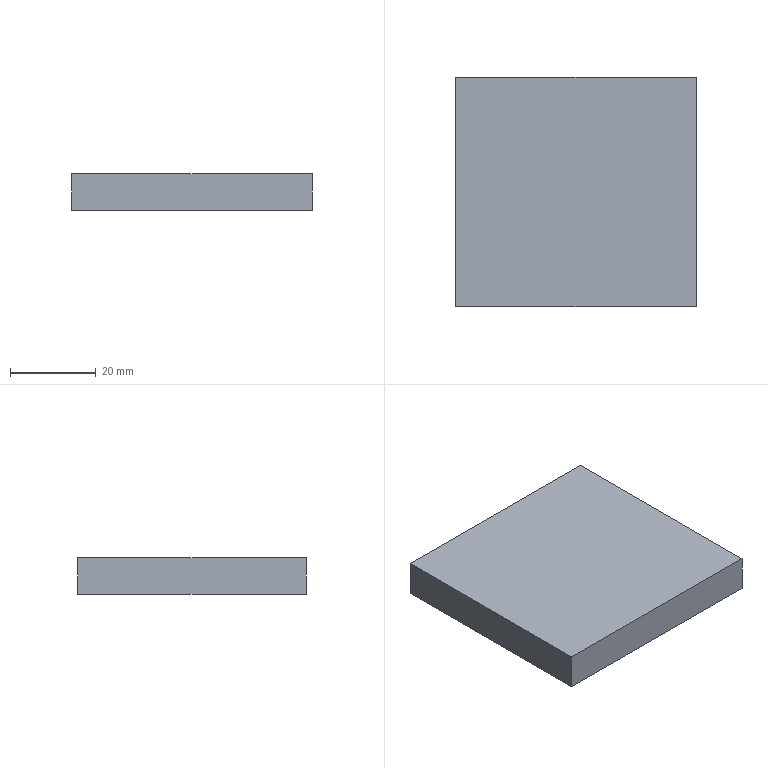NC program | NX | posted with a generic post | part box 56 x 53.3 x 8.5 mm
Lines 1 to 1399 of 2424:
N10 G17 G21 G94 G90
(FLOOR_WALL_COPY , TOOL : D80)
N12 T19 M6
N14 G54
N16 G17 G0 G90 X-73. Y0. S6500 M3
N18 G43 Z30. H19
N20 Z3.
N22 G94 G1 Z0. F1500.
N24 X-68.
N26 X68.
N28 X73.
N30 Z3.
N32 G0 Z30.
N34 M5
(DRILLING_COPY_1 , TOOL : D6A45)
N36 T01 M6
N38 G54
N40 G17 G0 G90 X-16. Y-10. S5000 M3
N42 G43 Z30. H1
N44 G94 G81 G98 Z-1. F350. R3.
N46 X-10.4 Y16.2
N48 X4.1 Y18.5
N50 X16. Y10.
N52 G80
N54 G0 X16. Y10. Z30.
N56 M5
(DRILLING_COPY_1_COPY , TOOL : 2.0ZT)
N58 T16 M6
N60 G54
N62 G17 G0 G90 X4.1 Y18.5 S2000 M3
N64 G43 Z30. H16
N66 G94 G83 G98 Z-3.101 F150. Q2. R3.
N68 X-10.4 Y16.2
N70 G80
N72 G0 X-10.4 Y16.2 Z30.
N74 M5
(DRILLING_COPY_1_COPY_COPY , TOOL : 2.4ZT)
N76 T17 M6
N78 G54
N80 G17 G0 G90 X-16. Y-10. S2000 M3
N82 G43 Z30. H17
N84 G94 G83 G98 Z-5.721 F150. Q2. R3.
N86 X16. Y10.
N88 G80
N90 G0 X16. Y10. Z30.
N92 M5
(ADAPTIVE_MILLING , TOOL : D10)
N94 T15 M6
N96 G54
N98 G17 G0 G90 X-35.709 Y0.039 S9500 M3
N100 G43 Z30. H15
N102 Z-0.5
N104 G94 G1 Z-3.5 F1000.
N106 X-34.928 Y-0.241 F3000.
N108 X-34.14 Y-0.497
N110 G3 X-33.062 Y0.039 R1.017
N112 X-32.301 Y3.102 R8.28
N114 X-32.018 Y12.969 R111.643
N116 G1 X-32.014 Y15.219
N118 X-32.011 Y19.094
N120 X-32.01 Y23.594
N122 X-32.005 Y23.844
N124 X-31.996 Y23.969
N126 X-31.983 Y24.093
N128 G2 X-29.126 Y28.303 R6.082
N130 X-23.363 Y30.215 R13.607
N132 X-14.877 Y30.613 R73.957
N134 G1 X-13.627 Y30.621
N136 X-12.127 Y30.628
N138 X-9.877 Y30.633
N140 X-6.252 Y30.636
N142 X4.748 Y30.638
N144 X24.998
N146 G2 X29.25 Y28.336 R5.606
N148 X31.446 Y22.821 R11.938
N150 X31.954 Y14.47 R57.249
N152 G1 X31.965 Y13.345
N154 X31.973 Y12.095
N156 X31.979 Y10.595
N158 X31.984 Y8.345
N160 X31.987 Y4.47
N162 X31.988 Y-9.155
N164 G2 X31.958 Y-24.154 R786.442
N166 X29.074 Y-28.344 R6.068
N168 X23.298 Y-30.225 R13.818
N170 X14.187 Y-30.618 R81.444
N172 G1 X12.937 Y-30.625
N174 X11.062 Y-30.631
N176 X8.312 Y-30.635
N178 X2.937 Y-30.637
N180 X-25.063 Y-30.638
N182 X-25.188 Y-30.635
N184 G2 X-29.515 Y-27.986 R5.827
N186 X-31.515 Y-22.387 R12.902
N188 X-31.964 Y-13.53 R68.549
N190 X-31.945 Y-2.656 R313.124
N192 G3 X-31.266 Y4.184 R246.26
N194 X-31.025 Y17.68 R253.193
N196 G2 X-30.938 Y21.676 R34.702
N198 X-26.882 Y27.245 R7.984
N200 X-20.34 Y29.196 R16.868
N202 X-10.728 Y29.602 R93.012
N204 G1 X-9.228 Y29.612
N206 X-7.728 Y29.618
N208 X-5.353 Y29.623
N210 X-1.353 Y29.626
N212 X11.272 Y29.627
N214 X21.897
N216 G2 X28.333 Y25.939 R7.618
N218 X30.48 Y19.467 R15.556
N220 X30.949 Y9.86 R80.002
N222 G1 X30.958 Y8.61
N224 X30.966 Y6.985
N226 X30.972 Y4.735
N228 X30.975 Y1.36
N230 X30.977 Y-6.39
N232 Y-20.515
N234 G2 X27.52 Y-26.824 R7.557
N236 X21.095 Y-29.096 R15.023
N238 X11.49 Y-29.597 R73.918
N240 G1 X10.24 Y-29.606
N242 X8.865 Y-29.613
N244 X6.865 Y-29.62
N246 X3.99 Y-29.624
N248 X-1.51 Y-29.626
N250 X-21.885 Y-29.627
N252 G2 X-28.186 Y-26.156 R7.552
N254 X-30.409 Y-19.974 R14.802
N256 X-30.94 Y-10.872 R67.194
N258 X-30.493 Y1.36 R90.695
N260 G3 X-30.042 Y17.349 R205.607
N262 G2 X-28.715 Y22.853 R9.591
N264 X-22.888 Y27.14 R10.859
N266 X-15.391 Y28.397 R28.546
N268 X-1.019 Y28.613 R293.42
N270 G1 X4.106 Y28.615
N272 X19.231 Y28.616
N274 X19.606 Y28.612
N276 X19.731 Y28.609
N278 X19.981 Y28.6
N280 X20.105 Y28.593
N282 G2 X27.438 Y23.856 R8.921
N284 X29.471 Y17.075 R18.202
N286 X29.936 Y7.092 R89.122
N288 G1 X29.946 Y5.842
N290 X29.954 Y4.217
N292 X29.959 Y2.217
N294 X29.964 Y-0.908
N296 X29.966 Y-6.908
N298 Y-17.908
N300 G2 X25.183 Y-26.102 R8.956
N302 X18.028 Y-28.173 R18.615
N304 X8.416 Y-28.587 R94.427
N306 G1 X7.041 Y-28.596
N308 X5.292 Y-28.604
N310 X3.042 Y-28.61
N312 X-0.458 Y-28.614
N314 X-7.833 Y-28.616
N316 X-19.208
N318 G2 X-27.427 Y-23.878 R8.94
N320 X-29.482 Y-16.976 R18.308
N322 X-29.583 Y-0.127 R88.532
N324 G3 X-29.046 Y16.236 R256.072
N326 G2 X-23.515 Y25.097 R9.923
N328 X-16.337 Y27.116 R20.252
N330 X-5.227 Y27.579 R107.451
N332 G1 X-3.727 Y27.588
N334 X-1.852 Y27.595
N336 X0.773 Y27.601
N338 X4.898 Y27.604
N340 X15.898 Y27.605
N342 X17.023
N344 G2 X23.681 Y25.524 R10.12
N346 X27.61 Y19.27 R12.456
N348 X28.753 Y11.497 R33.234
N350 X28.952 Y-3.25 R342.251
N352 X28.926 Y-16.75 R787.554
N354 X23.551 Y-25.057 R9.789
N356 X16.384 Y-27.111 R19.878
N358 X5.275 Y-27.58 R106.924
N360 G1 X3.775 Y-27.589
N362 X1.775 Y-27.596
N364 X-0.975 Y-27.601
N366 X-5.475 Y-27.604
N368 X-16.85 Y-27.605
N370 X-17.225 Y-27.603
N372 G2 X-26.465 Y-22.091 R9.883
N374 X-28.458 Y-15.033 R20.3
N376 X-28.662 Y-1.927 R74.071
N378 G3 X-28.053 Y14.684 R379.618
N380 G2 X-22. Y24.063 R10.638
N382 X-14.44 Y26.108 R21.789
N384 X-3.382 Y26.566 R113.181
N386 X2.387 Y26.68 R28.057
N388 G1 X3.011 Y26.665
N390 X3.636 Y26.654
N392 X4.511 Y26.643
N394 X5.636 Y26.634
N396 X7.136 Y26.627
N398 X9.136 Y26.621
N400 X12.261 Y26.618
N402 X14.011 Y26.616
N404 X14.761 Y26.611
N406 X15.261 Y26.605
N408 X15.511 Y26.6
N410 X15.761 Y26.593
N412 X16.136 Y26.577
N414 G2 X25.417 Y20.594 R10.522
N416 X27.462 Y13.035 R21.667
N418 X27.901 Y3.547 R101.721
N420 X28.033 Y-2.23 R26.861
N422 G1 X28.02 Y-2.73
N424 X28.007 Y-3.354
N426 X28. Y-3.854
N428 X27.989 Y-4.854
N430 X27.981 Y-6.104
N432 X27.974 Y-7.729
N434 X27.97 Y-10.104
N436 X27.967 Y-12.604
N438 X27.962 Y-13.354
N440 X27.954 Y-13.979
N442 X27.948 Y-14.229
N444 X27.935 Y-14.604
N446 X27.929 Y-14.729
N448 G2 X21.883 Y-24.101 R10.563
N450 X14.44 Y-26.105 R21.679
N452 X3.37 Y-26.568 R110.818
N454 X-2.387 Y-26.68 R28.095
N456 G1 X-3.011 Y-26.665
N458 X-3.636 Y-26.654
N460 X-4.511 Y-26.643
N462 X-5.636 Y-26.634
N464 X-7.136 Y-26.627
N466 X-9.136 Y-26.621
N468 X-12.261 Y-26.618
N470 X-14.011 Y-26.616
N472 X-14.761 Y-26.611
N474 X-15.261 Y-26.605
N476 X-15.511 Y-26.6
N478 X-15.886 Y-26.589
N480 X-16.136 Y-26.578
N482 G2 X-25.358 Y-20.705 R10.493
N484 X-27.449 Y-13.159 R21.481
N486 X-27.73 Y-4.617 R60.605
N488 G1 X-27.989 Y-2.991
N490 X-27.995 Y-2.935
N492 G2 X-27.556 Y5.706 R30.137
N494 G3 X-27.106 Y12.94 R98.432
N496 G2 X-24.212 Y20.348 R11.486
N498 X-17.228 Y24.284 R14.404
N500 X-8.567 Y25.4 R40.82
N502 G1 X-8.443 Y25.417
N504 X-5.945 Y26.131
N506 X-5.887 Y26.144
N508 X-3.299 Y26.58
N510 X-2.947 Y26.636
N512 X0.015 Y26.799
N514 X2.947 Y26.636
N516 X3.006 Y26.629
N518 G3 X8.799 Y25.803 R52.382
N520 G2 X15.168 Y25.547 R338.64
N522 X24.383 Y19.168 R11.095
N524 X26.43 Y11.477 R22.827
N526 G3 X26.7 Y8.869 R39.134
N528 G2 X27.904 Y3.531 R28.312
N530 G3 X29.234 Y2.749 R1.003
N532 X29.846 Y3.376 Z-3.455 R1.051
N534 G1 X30.288 Y4.378 Z-3.4
N536 X31.032 Y6.062
N538 G3 X31.086 Y6.713 R1.04
N540 G1 X28.465 Y17.012
N542 G3 X27.102 Y20.468 R15.003
N544 X24.439 Y24.532 R32.276
N546 X21.759 Y26.717 R9.19
N548 X18.514 Y27.978 R14.859
N550 X14.231 Y28.801 R25.607
N552 G1 X9.127 Y29.313
N554 X8.873 Y29.302
N556 X8.627 Y29.234
N558 X6.893 Y28.477
N560 X6.279 Y28.214 Z-3.433
N562 X5.674 Y27.93 Z-3.467
N564 G3 X5.274 Y27.417 Z-3.5 R1.041
N566 X5.945 Y26.131 R1.004
N568 X10.228 Y25.051 R31.02
N570 G2 X15.184 Y24.411 R63.089
N572 X23.404 Y17.715 R11.779
N574 X25.26 Y11.25 R23.658
N576 G3 X26.072 Y10.138 R3.622
N578 G1 X26.147 Y10.022
N580 X26.732 Y8.802
N582 G3 X28.202 Y8.411 R1.004
N584 X28.638 Y9.19 Z-3.454 R1.048
N586 G1 X28.79 Y10.256 Z-3.4
N588 X28.938 Y11.271
N590 X29.07 Y12.289
N592 X29.044 Y12.497
N594 X28.982 Y12.699
N596 X27.452 Y16.118
N598 X25.886 Y19.521
N600 G3 X24.53 Y21.596 R9.685
N602 G1 X22.082 Y24.428
N604 X21.658 Y24.883
N606 X21.198 Y25.302
N608 X20.679 Y25.645
N610 X20.136 Y25.949
N612 G3 X17.84 Y26.89 R10.567
N614 G1 X11.937 Y28.51
N616 G3 X11.231 Y28.443 R1.031
N618 G1 X9.669 Y27.675
N620 X9.076 Y27.39 Z-3.433
N622 X8.495 Y27.082 Z-3.466
N624 G3 X8.116 Y26.529 Z-3.5 R1.039
N626 X8.755 Y25.328 R1.005
N628 X13.562 Y23.782 R25.701
N630 G2 X22.775 Y15.535 R13.142
N632 G3 X23.994 Y12.123 R117.749
N634 X25.102 Y11.242 R3.94
N636 G1 X25.204 Y11.15
N638 X25.448 Y10.865
N640 G3 X26.99 Y10.892 R1.003
N642 X27.182 Y11.762 Z-3.454 R1.049
N644 G1 X27.021 Y12.829 Z-3.4
N646 X26.707 Y14.914
N648 X26.667 Y15.065
N650 X26.613 Y15.212
N652 X25.834 Y16.772
N654 X25.041 Y18.325
N656 G3 X22.137 Y22.189 R17.429
N658 G1 X20.539 Y23.766
N660 G3 X16.662 Y26.077 R11.549
N662 G1 X14.211 Y26.942
N664 X13.987 Y26.989
N666 X13.759 Y26.991
N668 X11.877 Y26.766
N670 X11.14 Y26.684 Z-3.437
N672 X10.406 Y26.574 Z-3.474
N674 X10.173 Y26.467 Z-3.487
N676 X9.971 Y26.308 Z-3.5
N678 G3 X10.314 Y24.692 R1.002
N680 G1 X11.514 Y24.199
N682 X11.567 Y24.173
N684 G2 X16.266 Y21.5 R63.352
N686 X21. Y16.103 R14.906
N688 X23.38 Y13.099 R9.472
N690 G1 X23.823 Y12.266
N692 X23.969 Y12.057
N694 X24.16 Y11.888
N696 X24.263 Y11.818
N698 G3 X25.693 Y13.472 R1.1
N700 G1 X15.529 Y24.444
N702 G3 X14.119 Y22.777 R-1.1
N704 G2 X16.403 Y20.608 R8.833
N706 X18.928 Y17.35 R100.947
N708 G3 X20.608 Y16.403 R30.815
N710 G1 X21.181 Y15.919
N712 G3 X22.66 Y17.546 R1.1
N714 G1 X18.08 Y22.015
N716 G3 X16.403 Y20.608 R1.1
N718 G2 X17.683 Y18.095 R38.392
N720 G3 X18.381 Y17.423 R1.477
N722 G1 X19.113 Y17.208
N724 X19.215 Y17.166
N726 G3 X20.37 Y18.999 R1.1
N728 G1 X19.001 Y20.238
N730 G3 X17.208 Y19.113 R1.101
N732 G1 X17.582 Y17.954
N734 G3 X18.437 Y17.406 R1.304
N736 X19.095 Y17.439 R1.04
N738 G1 X20.013 Y17.812
N740 X21.866 Y18.565 Z-3.4
N742 G2 X22.783 Y18.571 R1.049
N744 G1 X23.283 Y18.323
N746 X23.759 Y18.033
N748 X24.034 Y17.788
N750 X24.278 Y17.513
N752 X26.188 Y14.99
N754 X28.077 Y12.453
N756 G2 X30.648 Y6.937 R17.445
N758 X31.095 Y3.879 R15.296
N760 G1 X31.215 Y0.952
N762 G2 X30.666 Y0.01 R1.048
N764 G1 X29.002 Y-1.1 Z-3.5
N766 X28.355 Y-1.545
N768 G3 X28.033 Y-2.23 R1.028
N770 G2 X27.448 Y-6.278 R30.769
N772 G3 X26.997 Y-12.632 R51.118
N774 G2 X25.158 Y-19.035 R12.212
N776 X18.864 Y-23.751 R12.579
N778 X11.032 Y-25.252 R29.383
N780 G1 X10.658 Y-25.28
N782 X10.284 Y-25.306
N784 X9.785 Y-25.337
N786 X9.286 Y-25.365
N788 X8.786 Y-25.39
N790 X8.661 Y-25.396
N792 X8.537 Y-25.403
N794 X8.449 Y-25.415
N796 G2 X3.299 Y-26.58 R27.906
N798 G3 X2.533 Y-27.927 R1.003
N800 X3.244 Y-28.559 Z-3.451 R1.125
N802 G1 X4.179 Y-28.955 Z-3.4
N804 X5.116 Y-29.357
N806 X6.06 Y-29.742
N808 X6.269 Y-29.77
N810 X6.481 Y-29.762
N812 X9.278 Y-29.297
N814 X12.071 Y-28.815
N816 G3 X20.872 Y-26.306 R54.424
N818 X25.458 Y-23.284 R13.721
N820 G1 X27.126 Y-21.598
N822 G3 X29.12 Y-18.181 R10.513
N824 X29.834 Y-15.28 R15.037
N826 G1 X30.703 Y-9.092
N828 G3 X30.628 Y-8.55 R1.057
N830 G1 X29.876 Y-6.844
N832 X29.61 Y-6.229 Z-3.434
N834 X29.323 Y-5.623 Z-3.467
N836 G3 X28.813 Y-5.225 Z-3.5 R1.041
N838 X27.521 Y-5.91 R1.004
N840 X26.347 Y-10.792 R40.457
N842 G2 X25.123 Y-16.007 R19.384
N844 X18.615 Y-22.266 R12.231
N846 X11.982 Y-23.984 R24.516
N848 X8.394 Y-25.431 R37.714
N850 G3 X8.03 Y-27.162 R1.002
N852 X8.757 Y-27.406 Z-3.461 R1.195
N854 G1 X9.97 Y-27.526 Z-3.4
N856 X12.038 Y-27.722
N858 X12.291 Y-27.681
N860 G3 X16.749 Y-26.268 R69.932
N862 G1 X18.643 Y-25.538
N864 X20.527 Y-24.783
N866 G3 X27.746 Y-17.416 R14.045
N868 X29.948 Y-11.893 R86.613
N870 X29.895 Y-11.082 R1.025
N872 G1 X29.116 Y-9.599
N874 X28.817 Y-9.017 Z-3.433
N876 X28.495 Y-8.448 Z-3.465
N878 G3 X27.924 Y-8.083 Z-3.5 R1.038
N880 X26.766 Y-8.711 R1.005
N882 X25.065 Y-13.086 R28.708
N884 G2 X16.851 Y-21.453 R13.574
N886 G1 X14.951 Y-22.139
N888 X14.19 Y-22.73
N890 X14.119 Y-22.777
N892 X11.707 Y-24.097
N894 G3 X12.106 Y-25.971 R1.001
N896 G1 X12.43 Y-25.948 Z-3.484
N898 X12.749 Y-25.887 Z-3.468
N900 X14.076 Y-25.64 Z-3.4
N902 X16.053 Y-25.262
N904 X17.119 Y-24.908
N906 X18.168 Y-24.508
N908 X18.839 Y-24.181
N910 X19.489 Y-23.815
N912 X20.647 Y-23.102
N914 X21.777 Y-22.345
N916 G3 X27.102 Y-16.284 R18.483
N918 G1 X28.397 Y-13.92
N920 G3 X28.503 Y-13.256 R1.039
N922 G1 X28.177 Y-11.507
N924 X28.062 Y-10.861 Z-3.433
N926 X27.922 Y-10.22 Z-3.466
N928 G3 X27.488 Y-9.704 Z-3.5 R1.039
N930 X26.147 Y-10.022 R1.005
N932 X24.124 Y-13.185 R18.084
N934 G2 X16.965 Y-19.933 R15.92
N936 G3 X16.403 Y-20.608 R1.775
N938 G1 X15.448 Y-21.738
N940 X15.368 Y-21.814
N942 X14.875 Y-22.198
N944 G3 X16.354 Y-23.817 R-1.1
N946 G1 X27.386 Y-11.983
N948 G3 X25.746 Y-10.518 R-1.1
N950 G2 X24.367 Y-11.919 R13.436
N952 G3 X22.735 Y-14.183 R9.053
N954 G2 X19.689 Y-17.025 R9.403
N956 G3 X17.513 Y-18.488 R28.01
N958 X17.166 Y-19.215 R2.18
N960 G1 X16.574 Y-20.315
N962 G3 X18.309 Y-21.625 R1.1
N964 G1 X21.806 Y-18.222
N966 G3 X20.517 Y-16.465 R1.1
N968 G2 X18.282 Y-17.481 R9.189
N970 G3 X17.471 Y-18.215 R1.405
N972 G1 X17.26 Y-18.934
N974 G3 X19.197 Y-19.902 R1.1
N976 G1 X19.565 Y-19.416
N978 X19.916 Y-18.917
N980 G3 X18.633 Y-17.349 R1.101
N982 X17.582 Y-17.954 R1.573
N984 G1 X17.477 Y-18.197
N986 X17.441 Y-18.317
N988 G3 X19.231 Y-19.446 R1.101
N990 G1 X26.458 Y-12.969
N992 G3 X25.102 Y-11.242 R1.1
N994 G1 X23.969 Y-12.057
N996 X23.823 Y-12.266
N998 X23.412 Y-13.039
N1000 G3 X23.439 Y-14.024 R1.014
N1002 G1 X23.532 Y-14.178
N1004 X24.564 Y-15.891 Z-3.4
N1006 X24.73 Y-16.169
N1008 X24.848 Y-16.47
N1010 G2 X24.577 Y-17.385 R1.014
N1012 G1 X21.886 Y-20.084
N1014 X19.178 Y-22.767
N1016 G2 X10.914 Y-27.775 R24.066
N1018 G1 X9.243 Y-28.338
N1020 X7.564 Y-28.878
N1022 G2 X3.674 Y-29.635 R22.453
N1024 G1 X1.295 Y-29.877
N1026 G2 X0.281 Y-29.311 R1.044
N1028 G1 X-0.798 Y-27.627 Z-3.5
N1030 X-1.195 Y-27.029
N1032 G3 X-1.887 Y-26.695 R1.027
N1034 G1 X-2.947 Y-26.636
N1036 X-3.006 Y-26.629
N1038 G3 X-8.674 Y-25.811 R53.585
N1040 G2 X-15.168 Y-25.549 R437.385
N1042 X-24.325 Y-19.279 R11.081
N1044 X-26.445 Y-11.227 R22.473
N1046 G3 X-26.659 Y-8.954 R22.562
N1048 G2 X-27.747 Y-4.508 R24.302
N1050 G3 X-29.732 Y-4.592 R1.
N1052 G1 X-29.741 Y-4.718
N1054 X-29.887 Y-6.712 Z-3.4
N1056 X-29.955 Y-7.558
N1058 X-29.997 Y-8.405
N1060 G3 X-29.326 Y-13.344 R39.86
N1062 X-27.443 Y-19.93 R34.595
N1064 X-25.231 Y-23.66 R15.155
N1066 X-18.379 Y-27.992 R12.997
N1068 G1 X-17.336 Y-28.197
N1070 G3 X-9.127 Y-29.313 R190.173
N1072 X-8.606 Y-29.235 R1.064
N1074 G1 X-6.886 Y-28.478
N1076 X-6.274 Y-28.214 Z-3.433
N1078 X-5.671 Y-27.928 Z-3.467
N1080 G3 X-5.272 Y-27.411 Z-3.5 R1.04
N1082 X-5.945 Y-26.131 R1.004
N1084 X-10.305 Y-25.04 R30.615
N1086 G2 X-15.139 Y-24.424 R61.514
N1088 X-23.382 Y-17.756 R11.77
N1090 X-25.232 Y-11.292 R22.903
N1092 G1 X-25.27 Y-11.173
N1094 X-25.321 Y-11.058
N1096 X-25.383 Y-10.95
N1098 X-25.404 Y-10.917
N1100 G2 X-26.687 Y-8.895 R5.766
N1102 G3 X-28.155 Y-8.503 R1.004
N1104 X-28.593 Y-9.283 Z-3.454 R1.048
N1106 G1 X-28.745 Y-10.348 Z-3.4
N1108 X-28.893 Y-11.364
N1110 X-29.025 Y-12.382
N1112 X-28.999 Y-12.591
N1114 X-28.937 Y-12.792
N1116 X-27.407 Y-16.212
N1118 X-25.841 Y-19.615
N1120 G3 X-24.486 Y-21.689 R9.685
N1122 G1 X-22.911 Y-23.501
N1124 G3 X-17.068 Y-27.042 R12.903
N1126 G1 X-11.891 Y-28.523
N1128 G3 X-11.185 Y-28.464 R1.031
N1130 G1 X-9.592 Y-27.702
N1132 X-8.994 Y-27.421 Z-3.433
N1134 X-8.407 Y-27.119 Z-3.466
N1136 G3 X-8.022 Y-26.576 Z-3.5 R1.039
N1138 X-8.709 Y-25.341 R1.005
N1140 X-13.442 Y-23.818 R24.693
N1142 G2 X-22.722 Y-15.648 R13.1
N1144 G1 X-22.814 Y-15.416
N1146 X-22.904 Y-15.182
N1148 X-22.991 Y-14.948
N1150 X-23.075 Y-14.712
N1152 X-23.195 Y-14.357
N1154 X-23.234 Y-14.238
N1156 X-23.349 Y-13.881
N1158 X-23.425 Y-13.643
N1160 X-23.541 Y-13.287
N1162 X-23.621 Y-13.05
N1164 X-23.662 Y-12.932
N1166 X-23.746 Y-12.696
N1168 X-23.789 Y-12.579
N1170 X-23.835 Y-12.462
N1172 X-23.881 Y-12.346
N1174 X-23.929 Y-12.231
N1176 X-24.234 Y-11.838
N1178 G2 X-25.448 Y-10.865 R4.616
N1180 G3 X-26.99 Y-10.892 R1.003
N1182 X-27.182 Y-11.762 Z-3.454 R1.049
N1184 G1 X-27.021 Y-12.829 Z-3.4
N1186 X-26.707 Y-14.914
N1188 X-26.667 Y-15.065
N1190 X-26.613 Y-15.212
N1192 X-25.834 Y-16.772
N1194 X-25.041 Y-18.325
N1196 G3 X-22.137 Y-22.189 R17.429
N1198 G1 X-20.539 Y-23.766
N1200 G3 X-16.662 Y-26.077 R11.549
N1202 G1 X-14.211 Y-26.942
N1204 X-13.987 Y-26.989
N1206 X-13.759 Y-26.991
N1208 X-11.877 Y-26.766
N1210 X-11.14 Y-26.684 Z-3.437
N1212 X-10.406 Y-26.574 Z-3.474
N1214 X-10.173 Y-26.467 Z-3.487
N1216 X-9.971 Y-26.308 Z-3.5
N1218 G3 X-10.314 Y-24.692 R1.002
N1220 G1 X-11.514 Y-24.199
N1222 X-11.567 Y-24.173
N1224 G2 X-16.37 Y-21.43 R58.634
N1226 X-20.997 Y-16.101 R15.088
N1228 X-23.38 Y-13.099 R9.355
N1230 G1 X-23.823 Y-12.266
N1232 X-23.969 Y-12.057
N1234 X-24.16 Y-11.888
N1236 X-24.263 Y-11.818
N1238 G3 X-25.693 Y-13.472 R1.1
N1240 G1 X-15.529 Y-24.444
N1242 G3 X-14.119 Y-22.777 R-1.1
N1244 G2 X-16.403 Y-20.608 R8.833
N1246 X-18.926 Y-17.349 R135.852
N1248 G3 X-20.608 Y-16.403 R40.938
N1250 G1 X-21.086 Y-15.999
N1252 G3 X-22.565 Y-17.625 R1.1
N1254 G1 X-18.081 Y-22.014
N1256 G3 X-16.403 Y-20.608 R1.1
N1258 G2 X-17.684 Y-18.095 R39.38
N1260 G3 X-18.377 Y-17.424 R1.455
N1262 G1 X-19.113 Y-17.208
N1264 X-19.215 Y-17.166
N1266 G3 X-20.37 Y-18.999 R1.1
N1268 G1 X-19.001 Y-20.238
N1270 G3 X-17.208 Y-19.113 R1.101
N1272 G1 X-17.582 Y-17.954
N1274 G3 X-18.437 Y-17.406 R1.304
N1276 X-19.095 Y-17.439 R1.04
N1278 G1 X-20.013 Y-17.812
N1280 X-21.866 Y-18.565 Z-3.4
N1282 G2 X-22.783 Y-18.571 R1.049
N1284 G1 X-23.283 Y-18.323
N1286 X-23.759 Y-18.033
N1288 X-24.034 Y-17.788
N1290 X-24.278 Y-17.513
N1292 X-28.04 Y-12.525
N1294 G2 X-29.751 Y-9.255 R11.428
N1296 X-30.79 Y-5.79 R49.946
N1298 X-31.067 Y-3.82 R12.101
N1300 G1 X-31.453 Y3.456
N1302 G2 X-30.623 Y4.495 R1.005
N1304 G1 X-30.293 Y4.551
N1306 X-28.321 Y4.889 Z-3.5
N1308 G3 X-27.556 Y5.706 R1.01
N1310 X-26.566 Y9.803 R55.236
N1312 G2 X-25.727 Y14.599 R35.042
N1314 X-18.923 Y22.156 R12.05
N1316 X-11.94 Y24. R24.418
N1318 X-8.394 Y25.431 R36.809
N1320 G3 X-8.03 Y27.162 R1.002
N1322 X-8.757 Y27.406 Z-3.461 R1.195
N1324 G1 X-9.97 Y27.526 Z-3.4
N1326 X-12.038 Y27.722
N1328 X-12.291 Y27.681
N1330 G3 X-16.749 Y26.268 R69.932
N1332 G1 X-18.392 Y25.634
N1334 X-20.028 Y24.979
N1336 G3 X-23.706 Y22.846 R19.002
N1338 G1 X-25.033 Y21.845
N1340 G3 X-26.664 Y19.889 R7.475
N1342 X-27.543 Y18.103 R12.651
N1344 G1 X-28.636 Y15.331
N1346 X-29.693 Y12.545
N1348 X-29.884 Y12.016
N1350 X-30.058 Y11.482
N1352 G3 X-29.972 Y10.858 R1.043
N1354 G1 X-29.212 Y9.317
N1356 X-28.922 Y8.718 Z-3.433
N1358 X-28.611 Y8.13 Z-3.467
N1360 G3 X-28.074 Y7.753 Z-3.5 R1.04
N1362 X-26.835 Y8.454 R1.004
N1364 G2 X-26.102 Y10.163 R14.753
N1366 X-24.552 Y14.517 R53.806
N1368 X-16.881 Y21.47 R13.551
N1370 G3 X-14.897 Y22.18 R38.687
N1372 G1 X-14.19 Y22.73
N1374 X-14.119 Y22.777
N1376 X-11.707 Y24.097
N1378 G3 X-12.106 Y25.971 R1.001
N1380 G1 X-12.43 Y25.948 Z-3.484
N1382 X-12.749 Y25.887 Z-3.468
N1384 X-14.076 Y25.64 Z-3.4
N1386 X-16.053 Y25.262
N1388 X-17.119 Y24.908
N1390 X-18.168 Y24.508
N1392 X-18.839 Y24.181
N1394 X-19.489 Y23.815
N1396 X-22.097 Y22.19
N1398 G3 X-26.534 Y17.306 R14.088
N1400 G1 X-28.496 Y13.713
N1402 G3 X-28.606 Y13.078 R1.041
N1404 G1 X-28.322 Y11.278
N1406 X-28.221 Y10.606 Z-3.434
N1408 X-28.098 Y9.937 Z-3.468
N1410 G3 X-27.724 Y9.432 Z-3.5 R1.043
N1412 X-26.246 Y9.816 R1.004
N1414 G2 X-25.464 Y10.931 R9.583
N1416 X-23.163 Y14.796 R75.329
N1418 X-16.889 Y20.008 R16.055
N1420 G3 X-16.403 Y20.608 R1.949
N1422 G1 X-15.448 Y21.738
N1424 X-15.368 Y21.814
N1426 X-14.875 Y22.198
N1428 G3 X-16.354 Y23.816 R-1.1
N1430 G1 X-27.468 Y11.888
N1432 G3 X-25.828 Y10.423 R-1.1
N1434 G2 X-24.296 Y12.025 R20.803
N1436 G3 X-22.735 Y14.183 R9.034
N1438 G2 X-20.004 Y16.822 R9.165
N1440 G3 X-17.519 Y18.498 R44.358
N1442 X-17.166 Y19.215 R2.054
N1444 G1 X-16.514 Y20.425
N1446 G3 X-18.256 Y21.729 R1.1
N1448 G1 X-21.812 Y18.216
N1450 G3 X-20.517 Y16.465 R1.1
N1452 G2 X-18.283 Y17.482 R9.282
N1454 G3 X-17.47 Y18.219 R1.421
N1456 G1 X-17.259 Y18.938
N1458 G3 X-19.197 Y19.905 R1.1
N1460 G1 X-19.565 Y19.416
N1462 X-19.916 Y18.916
N1464 G3 X-18.633 Y17.349 R1.101
N1466 X-17.582 Y17.954 R1.573
N1468 G1 X-17.477 Y18.197
N1470 X-17.441 Y18.317
N1472 G3 X-19.231 Y19.446 R1.101
N1474 G1 X-26.458 Y12.969
N1476 G3 X-25.102 Y11.242 R1.1
N1478 G1 X-23.969 Y12.057
N1480 X-23.823 Y12.266
N1482 X-23.38 Y13.099
N1484 G3 X-23.917 Y14.518 R1.014
N1486 G1 X-25.164 Y14.987
N1488 Z-0.5
N1490 G0 Z30.
N1492 M5
(ZLEVEL_PROFILE , TOOL : D4)
N1494 T11 M6
N1496 G54
N1498 G17 G0 G90 X-15.177 Y-17.833 S9500 M3
N1500 G43 Z30. H11
N1502 Z-0.389
N1504 G94 G1 X-14.683 Y-17.419 F1000.
N1506 G3 X-14.547 Y-17.043 R0.4
N1508 G2 X-14.098 Y-14.165 R4.5 F1650.
N1510 G1 X-14.072 Y-14.116
N1512 X-14.116 Y-14.072
N1514 X-14.165 Y-14.098
N1516 G2 X-17.043 Y-14.547 R4.5
N1518 G3 X-17.419 Y-14.683 R0.4
N1520 G1 X-17.833 Y-15.177
N1522 G0 X-15.177 Y-17.833 Z-0.778
N1524 G1 X-14.683 Y-17.419 F1000.
N1526 G3 X-14.547 Y-17.043 R0.4
N1528 G2 X-14.098 Y-14.165 R4.5 F1650.
N1530 G1 X-14.072 Y-14.116
N1532 X-14.116 Y-14.072
N1534 X-14.165 Y-14.098
N1536 G2 X-17.043 Y-14.547 R4.5
N1538 G3 X-17.419 Y-14.683 R0.4
N1540 G1 X-17.833 Y-15.177
N1542 G0 X-15.177 Y-17.833 Z-1.167
N1544 G1 X-14.683 Y-17.419 F1000.
N1546 G3 X-14.547 Y-17.043 R0.4
N1548 G2 X-14.098 Y-14.165 R4.5 F1650.
N1550 G1 X-14.072 Y-14.116
N1552 X-14.116 Y-14.072
N1554 X-14.165 Y-14.098
N1556 G2 X-17.043 Y-14.547 R4.5
N1558 G3 X-17.419 Y-14.683 R0.4
N1560 G1 X-17.833 Y-15.177
N1562 G0 X-15.177 Y-17.833 Z-1.556
N1564 G1 X-14.683 Y-17.419 F1000.
N1566 G3 X-14.547 Y-17.043 R0.4
N1568 G2 X-14.098 Y-14.165 R4.5 F1650.
N1570 G1 X-14.072 Y-14.116
N1572 X-14.116 Y-14.072
N1574 X-14.165 Y-14.098
N1576 G2 X-17.043 Y-14.547 R4.5
N1578 G3 X-17.419 Y-14.683 R0.4
N1580 G1 X-17.833 Y-15.177
N1582 G0 X-15.177 Y-17.833 Z-1.944
N1584 G1 X-14.683 Y-17.419 F1000.
N1586 G3 X-14.547 Y-17.043 R0.4
N1588 G2 X-14.098 Y-14.165 R4.5 F1650.
N1590 G1 X-14.072 Y-14.116
N1592 X-14.116 Y-14.072
N1594 X-14.165 Y-14.098
N1596 G2 X-17.043 Y-14.547 R4.5
N1598 G3 X-17.419 Y-14.683 R0.4
N1600 G1 X-17.833 Y-15.177
N1602 G0 X-15.172 Y-17.848 Z-2.333
N1604 G1 X-14.68 Y-17.433 F1000.
N1606 G3 X-14.544 Y-17.056 R0.4
N1608 G2 X-14.098 Y-14.165 R4.5 F1650.
N1610 G1 X-14.072 Y-14.116
N1612 X-14.116 Y-14.072
N1614 X-14.165 Y-14.098
N1616 G2 X-17.05 Y-14.546 R4.5
N1618 G3 X-17.426 Y-14.682 R0.4
N1620 G1 X-17.841 Y-15.174
N1622 G0 X-15.172 Y-17.848 Z-2.722
N1624 G1 X-14.68 Y-17.433 F1000.
N1626 G3 X-14.544 Y-17.056 R0.4
N1628 G2 X-14.098 Y-14.165 R4.5 F1650.
N1630 G1 X-14.072 Y-14.116
N1632 X-14.116 Y-14.072
N1634 X-14.165 Y-14.098
N1636 G2 X-17.05 Y-14.546 R4.5
N1638 G3 X-17.426 Y-14.682 R0.4
N1640 G1 X-17.841 Y-15.174
N1642 G0 X-15.172 Y-17.848 Z-3.111
N1644 G1 X-14.68 Y-17.433 F1000.
N1646 G3 X-14.544 Y-17.056 R0.4
N1648 G2 X-14.098 Y-14.165 R4.5 F1650.
N1650 G1 X-14.072 Y-14.116
N1652 X-14.116 Y-14.072
N1654 X-14.165 Y-14.098
N1656 G2 X-17.05 Y-14.546 R4.5
N1658 G3 X-17.426 Y-14.682 R0.4
N1660 G1 X-17.841 Y-15.174
N1662 G0 X-15.172 Y-17.848 Z-3.5
N1664 G1 X-14.68 Y-17.433 F1000.
N1666 G3 X-14.544 Y-17.056 R0.4
N1668 G2 X-14.098 Y-14.165 R4.5 F1650.
N1670 G1 X-14.072 Y-14.116
N1672 X-14.116 Y-14.072
N1674 X-14.165 Y-14.098
N1676 G2 X-17.05 Y-14.546 R4.5
N1678 G3 X-17.426 Y-14.682 R0.4
N1680 G1 X-17.841 Y-15.174
N1682 G0 Z30.
N1684 X-21.583 Y-11.488
N1686 Z-0.389
N1688 G1 X-21.206 Y-10.92 F1000.
N1690 G3 X-21.181 Y-10.521 R0.4
N1692 G2 X-21.665 Y-9.484 R23.65 F1650.
N1694 X-22.58 Y-9.195 R2.5
N1696 G3 X-22.98 Y-9.205 R0.4
N1698 G1 X-23.507 Y-9.526
N1700 G0 X-21.583 Y-11.488 Z-0.778
N1702 G1 X-21.206 Y-10.92 F1000.
N1704 G3 X-21.181 Y-10.521 R0.4
N1706 G2 X-21.665 Y-9.484 R23.65 F1650.
N1708 X-22.58 Y-9.195 R2.5
N1710 G3 X-22.98 Y-9.205 R0.4
N1712 G1 X-23.507 Y-9.526
N1714 G0 X-21.583 Y-11.488 Z-1.167
N1716 G1 X-21.206 Y-10.92 F1000.
N1718 G3 X-21.181 Y-10.521 R0.4
N1720 G2 X-21.665 Y-9.484 R23.65 F1650.
N1722 X-22.58 Y-9.195 R2.5
N1724 G3 X-22.98 Y-9.205 R0.4
N1726 G1 X-23.507 Y-9.526
N1728 G0 X-21.583 Y-11.488 Z-1.556
N1730 G1 X-21.206 Y-10.92 F1000.
N1732 G3 X-21.181 Y-10.521 R0.4
N1734 G2 X-21.665 Y-9.484 R23.65 F1650.
N1736 X-22.58 Y-9.195 R2.5
N1738 G3 X-22.98 Y-9.205 R0.4
N1740 G1 X-23.507 Y-9.526
N1742 G0 X-21.583 Y-11.488 Z-1.944
N1744 G1 X-21.206 Y-10.92 F1000.
N1746 G3 X-21.181 Y-10.521 R0.4
N1748 G2 X-21.665 Y-9.484 R23.65 F1650.
N1750 X-22.58 Y-9.195 R2.5
N1752 G3 X-22.98 Y-9.205 R0.4
N1754 G1 X-23.507 Y-9.526
N1756 G0 X-21.584 Y-11.486 Z-2.333
N1758 G1 X-21.207 Y-10.919 F1000.
N1760 G3 X-21.182 Y-10.519 R0.4
N1762 G2 X-21.665 Y-9.484 R23.65 F1650.
N1764 X-22.579 Y-9.195 R2.5
N1766 G3 X-22.979 Y-9.205 R0.4
N1768 G1 X-23.506 Y-9.527
N1770 G0 X-21.584 Y-11.486 Z-2.722
N1772 G1 X-21.207 Y-10.919 F1000.
N1774 G3 X-21.182 Y-10.519 R0.4
N1776 G2 X-21.665 Y-9.484 R23.65 F1650.
N1778 X-22.579 Y-9.195 R2.5
N1780 G3 X-22.979 Y-9.205 R0.4
N1782 G1 X-23.506 Y-9.527
N1784 G0 X-21.584 Y-11.486 Z-3.111
N1786 G1 X-21.207 Y-10.919 F1000.
N1788 G3 X-21.182 Y-10.519 R0.4
N1790 G2 X-21.665 Y-9.484 R23.65 F1650.
N1792 X-22.579 Y-9.195 R2.5
N1794 G3 X-22.979 Y-9.205 R0.4
N1796 G1 X-23.506 Y-9.527
N1798 G0 X-21.584 Y-11.486 Z-3.5
N1800 G1 X-21.207 Y-10.919 F1000.
N1802 G3 X-21.182 Y-10.519 R0.4
N1804 G2 X-21.665 Y-9.484 R23.65 F1650.
N1806 X-22.579 Y-9.195 R2.5
N1808 G3 X-22.979 Y-9.205 R0.4
N1810 G1 X-23.506 Y-9.527
N1812 G0 Z30.
N1814 X-23.507 Y9.526
N1816 Z-0.389
N1818 G1 X-22.98 Y9.204 F1000.
N1820 G3 X-22.58 Y9.195 R0.4
N1822 G2 X-21.665 Y9.484 R2.5 F1650.
N1824 X-21.181 Y10.521 R23.65
N1826 G3 X-21.206 Y10.92 R0.4
N1828 G1 X-21.583 Y11.488
N1830 G0 X-23.507 Y9.526 Z-0.778
N1832 G1 X-22.98 Y9.204 F1000.
N1834 G3 X-22.58 Y9.195 R0.4
N1836 G2 X-21.665 Y9.484 R2.5 F1650.
N1838 X-21.181 Y10.521 R23.65
N1840 G3 X-21.206 Y10.92 R0.4
N1842 G1 X-21.583 Y11.488
N1844 G0 X-23.507 Y9.526 Z-1.167
N1846 G1 X-22.98 Y9.204 F1000.
N1848 G3 X-22.58 Y9.195 R0.4
N1850 G2 X-21.665 Y9.484 R2.5 F1650.
N1852 X-21.181 Y10.521 R23.65
N1854 G3 X-21.206 Y10.92 R0.4
N1856 G1 X-21.583 Y11.488
N1858 G0 X-23.507 Y9.526 Z-1.556
N1860 G1 X-22.98 Y9.204 F1000.
N1862 G3 X-22.58 Y9.195 R0.4
N1864 G2 X-21.665 Y9.484 R2.5 F1650.
N1866 X-21.181 Y10.521 R23.65
N1868 G3 X-21.206 Y10.92 R0.4
N1870 G1 X-21.583 Y11.488
N1872 G0 X-23.507 Y9.526 Z-1.944
N1874 G1 X-22.98 Y9.204 F1000.
N1876 G3 X-22.58 Y9.195 R0.4
N1878 G2 X-21.665 Y9.484 R2.5 F1650.
N1880 X-21.181 Y10.521 R23.65
N1882 G3 X-21.206 Y10.92 R0.4
N1884 G1 X-21.583 Y11.488
N1886 G0 X-23.506 Y9.527 Z-2.333
N1888 G1 X-22.979 Y9.205 F1000.
N1890 G3 X-22.579 Y9.195 R0.4
N1892 G2 X-21.665 Y9.484 R2.5 F1650.
N1894 X-21.182 Y10.519 R23.65
N1896 G3 X-21.207 Y10.919 R0.4
N1898 G1 X-21.584 Y11.486
N1900 G0 X-23.506 Y9.527 Z-2.722
N1902 G1 X-22.979 Y9.205 F1000.
N1904 G3 X-22.579 Y9.195 R0.4
N1906 G2 X-21.665 Y9.484 R2.5 F1650.
N1908 X-21.182 Y10.519 R23.65
N1910 G3 X-21.207 Y10.919 R0.4
N1912 G1 X-21.584 Y11.486
N1914 G0 X-23.506 Y9.527 Z-3.111
N1916 G1 X-22.979 Y9.205 F1000.
N1918 G3 X-22.579 Y9.195 R0.4
N1920 G2 X-21.665 Y9.484 R2.5 F1650.
N1922 X-21.182 Y10.519 R23.65
N1924 G3 X-21.207 Y10.919 R0.4
N1926 G1 X-21.584 Y11.486
N1928 G0 X-23.506 Y9.527 Z-3.5
N1930 G1 X-22.979 Y9.205 F1000.
N1932 G3 X-22.579 Y9.195 R0.4
N1934 G2 X-21.665 Y9.484 R2.5 F1650.
N1936 X-21.182 Y10.519 R23.65
N1938 G3 X-21.207 Y10.919 R0.4
N1940 G1 X-21.584 Y11.486
N1942 G0 Z30.
N1944 X-17.833 Y15.177
N1946 Z-0.389
N1948 G1 X-17.419 Y14.683 F1000.
N1950 G3 X-17.043 Y14.547 R0.4
N1952 G2 X-14.165 Y14.098 R4.5 F1650.
N1954 G1 X-14.116 Y14.072
N1956 X-14.072 Y14.116
N1958 X-14.098 Y14.165
N1960 G2 X-14.547 Y17.043 R4.5
N1962 G3 X-14.683 Y17.419 R0.4
N1964 G1 X-15.177 Y17.833
N1966 G0 X-17.833 Y15.177 Z-0.778
N1968 G1 X-17.419 Y14.683 F1000.
N1970 G3 X-17.043 Y14.547 R0.4
N1972 G2 X-14.165 Y14.098 R4.5 F1650.
N1974 G1 X-14.116 Y14.072
N1976 X-14.072 Y14.116
N1978 X-14.098 Y14.165
N1980 G2 X-14.547 Y17.043 R4.5
N1982 G3 X-14.683 Y17.419 R0.4
N1984 G1 X-15.177 Y17.833
N1986 G0 X-17.833 Y15.177 Z-1.167
N1988 G1 X-17.419 Y14.683 F1000.
N1990 G3 X-17.043 Y14.547 R0.4
N1992 G2 X-14.165 Y14.098 R4.5 F1650.
N1994 G1 X-14.116 Y14.072
N1996 X-14.072 Y14.116
N1998 X-14.098 Y14.165
N2000 G2 X-14.547 Y17.043 R4.5
N2002 G3 X-14.683 Y17.419 R0.4
N2004 G1 X-15.177 Y17.833
N2006 G0 X-17.833 Y15.177 Z-1.556
N2008 G1 X-17.419 Y14.683 F1000.
N2010 G3 X-17.043 Y14.547 R0.4
N2012 G2 X-14.165 Y14.098 R4.5 F1650.
N2014 G1 X-14.116 Y14.072
N2016 X-14.072 Y14.116
N2018 X-14.098 Y14.165
N2020 G2 X-14.547 Y17.043 R4.5
N2022 G3 X-14.683 Y17.419 R0.4
N2024 G1 X-15.177 Y17.833
N2026 G0 X-17.833 Y15.177 Z-1.944
N2028 G1 X-17.419 Y14.683 F1000.
N2030 G3 X-17.043 Y14.547 R0.4
N2032 G2 X-14.165 Y14.098 R4.5 F1650.
N2034 G1 X-14.116 Y14.072
N2036 X-14.072 Y14.116
N2038 X-14.098 Y14.165
N2040 G2 X-14.547 Y17.043 R4.5
N2042 G3 X-14.683 Y17.419 R0.4
N2044 G1 X-15.177 Y17.833
N2046 G0 X-17.841 Y15.174 Z-2.333
N2048 G1 X-17.426 Y14.682 F1000.
N2050 G3 X-17.05 Y14.546 R0.4
N2052 G2 X-14.165 Y14.098 R4.5 F1650.
N2054 G1 X-14.116 Y14.072
N2056 X-14.072 Y14.116
N2058 X-14.098 Y14.165
N2060 G2 X-14.544 Y17.056 R4.5
N2062 G3 X-14.68 Y17.433 R0.4
N2064 G1 X-15.172 Y17.848
N2066 G0 X-17.841 Y15.174 Z-2.722
N2068 G1 X-17.426 Y14.682 F1000.
N2070 G3 X-17.05 Y14.546 R0.4
N2072 G2 X-14.165 Y14.098 R4.5 F1650.
N2074 G1 X-14.116 Y14.072
N2076 X-14.072 Y14.116
N2078 X-14.098 Y14.165
N2080 G2 X-14.544 Y17.056 R4.5
N2082 G3 X-14.68 Y17.433 R0.4
N2084 G1 X-15.172 Y17.848
N2086 G0 X-17.841 Y15.174 Z-3.111
N2088 G1 X-17.426 Y14.682 F1000.
N2090 G3 X-17.05 Y14.546 R0.4
N2092 G2 X-14.165 Y14.098 R4.5 F1650.
N2094 G1 X-14.116 Y14.072
N2096 X-14.072 Y14.116
N2098 X-14.098 Y14.165
N2100 G2 X-14.544 Y17.056 R4.5
N2102 G3 X-14.68 Y17.433 R0.4
N2104 G1 X-15.172 Y17.848
N2106 G0 X-17.841 Y15.174 Z-3.5
N2108 G1 X-17.426 Y14.682 F1000.
N2110 G3 X-17.05 Y14.546 R0.4
N2112 G2 X-14.165 Y14.098 R4.5 F1650.
N2114 G1 X-14.116 Y14.072
N2116 X-14.072 Y14.116
N2118 X-14.098 Y14.165
N2120 G2 X-14.544 Y17.056 R4.5
N2122 G3 X-14.68 Y17.433 R0.4
N2124 G1 X-15.172 Y17.848
N2126 G0 Z30.
N2128 X15.177 Y17.833
N2130 Z-0.389
N2132 G1 X14.683 Y17.419 F1000.
N2134 G3 X14.547 Y17.043 R0.4
N2136 G2 X14.098 Y14.165 R4.5 F1650.
N2138 G1 X14.072 Y14.116
N2140 X14.116 Y14.072
N2142 X14.165 Y14.098
N2144 G2 X17.043 Y14.547 R4.5
N2146 G3 X17.419 Y14.683 R0.4
N2148 G1 X17.833 Y15.177
N2150 G0 X15.177 Y17.833 Z-0.778
N2152 G1 X14.683 Y17.419 F1000.
N2154 G3 X14.547 Y17.043 R0.4
N2156 G2 X14.098 Y14.165 R4.5 F1650.
N2158 G1 X14.072 Y14.116
N2160 X14.116 Y14.072
N2162 X14.165 Y14.098
N2164 G2 X17.043 Y14.547 R4.5
N2166 G3 X17.419 Y14.683 R0.4
N2168 G1 X17.833 Y15.177
N2170 G0 X15.177 Y17.833 Z-1.167
N2172 G1 X14.683 Y17.419 F1000.
N2174 G3 X14.547 Y17.043 R0.4
N2176 G2 X14.098 Y14.165 R4.5 F1650.
N2178 G1 X14.072 Y14.116
N2180 X14.116 Y14.072
N2182 X14.165 Y14.098
N2184 G2 X17.043 Y14.547 R4.5
N2186 G3 X17.419 Y14.683 R0.4
N2188 G1 X17.833 Y15.177
N2190 G0 X15.177 Y17.833 Z-1.556
N2192 G1 X14.683 Y17.419 F1000.
N2194 G3 X14.547 Y17.043 R0.4
N2196 G2 X14.098 Y14.165 R4.5 F1650.
N2198 G1 X14.072 Y14.116
N2200 X14.116 Y14.072
N2202 X14.165 Y14.098
N2204 G2 X17.043 Y14.547 R4.5
N2206 G3 X17.419 Y14.683 R0.4
N2208 G1 X17.833 Y15.177
N2210 G0 X15.177 Y17.833 Z-1.944
N2212 G1 X14.683 Y17.419 F1000.
N2214 G3 X14.547 Y17.043 R0.4
N2216 G2 X14.098 Y14.165 R4.5 F1650.
N2218 G1 X14.072 Y14.116
N2220 X14.116 Y14.072
N2222 X14.165 Y14.098
N2224 G2 X17.043 Y14.547 R4.5
N2226 G3 X17.419 Y14.683 R0.4
N2228 G1 X17.833 Y15.177
N2230 G0 X15.176 Y17.834 Z-2.333
N2232 G1 X14.683 Y17.42 F1000.
N2234 G3 X14.547 Y17.044 R0.4
N2236 G2 X14.098 Y14.165 R4.5 F1650.
N2238 G1 X14.072 Y14.116
N2240 X14.116 Y14.072
N2242 X14.165 Y14.098
N2244 G2 X17.05 Y14.546 R4.5
N2246 G3 X17.426 Y14.682 R0.4
N2248 G1 X17.841 Y15.174
N2250 G0 X15.176 Y17.834 Z-2.722
N2252 G1 X14.683 Y17.42 F1000.
N2254 G3 X14.547 Y17.044 R0.4
N2256 G2 X14.098 Y14.165 R4.5 F1650.
N2258 G1 X14.072 Y14.116
N2260 X14.116 Y14.072
N2262 X14.165 Y14.098
N2264 G2 X17.05 Y14.546 R4.5
N2266 G3 X17.426 Y14.682 R0.4
N2268 G1 X17.841 Y15.174
N2270 G0 X15.176 Y17.834 Z-3.111
N2272 G1 X14.683 Y17.42 F1000.
N2274 G3 X14.547 Y17.044 R0.4
N2276 G2 X14.098 Y14.165 R4.5 F1650.
N2278 G1 X14.072 Y14.116
N2280 X14.116 Y14.072
N2282 X14.165 Y14.098
N2284 G2 X17.05 Y14.546 R4.5
N2286 G3 X17.426 Y14.682 R0.4
N2288 G1 X17.841 Y15.174
N2290 G0 X15.176 Y17.834 Z-3.5
N2292 G1 X14.683 Y17.42 F1000.
N2294 G3 X14.547 Y17.044 R0.4
N2296 G2 X14.098 Y14.165 R4.5 F1650.
N2298 G1 X14.072 Y14.116
N2300 X14.116 Y14.072
N2302 X14.165 Y14.098
N2304 G2 X17.05 Y14.546 R4.5
N2306 G3 X17.426 Y14.682 R0.4
N2308 G1 X17.841 Y15.174
N2310 G0 Z30.
N2312 X21.583 Y11.489
N2314 Z-0.389
N2316 G1 X21.206 Y10.921 F1000.
N2318 G3 X21.181 Y10.522 R0.4
N2320 G2 X21.665 Y9.484 R23.65 F1650.
N2322 X22.582 Y9.194 R2.5
N2324 G3 X22.982 Y9.203 R0.4
N2326 G1 X23.509 Y9.525
N2328 G0 X21.583 Y11.489 Z-0.778
N2330 G1 X21.206 Y10.921 F1000.
N2332 G3 X21.181 Y10.522 R0.4
N2334 G2 X21.665 Y9.484 R23.65 F1650.
N2336 X22.582 Y9.194 R2.5
N2338 G3 X22.982 Y9.203 R0.4
N2340 G1 X23.509 Y9.525
N2342 G0 X21.583 Y11.489 Z-1.167
N2344 G1 X21.206 Y10.921 F1000.
N2346 G3 X21.181 Y10.522 R0.4
N2348 G2 X21.665 Y9.484 R23.65 F1650.
N2350 X22.582 Y9.194 R2.5
N2352 G3 X22.982 Y9.203 R0.4
N2354 G1 X23.509 Y9.525
N2356 G0 X21.583 Y11.489 Z-1.556
N2358 G1 X21.206 Y10.921 F1000.
N2360 G3 X21.181 Y10.522 R0.4
N2362 G2 X21.665 Y9.484 R23.65 F1650.
N2364 X22.582 Y9.194 R2.5
N2366 G3 X22.982 Y9.203 R0.4
N2368 G1 X23.509 Y9.525
N2370 G0 X21.583 Y11.489 Z-1.944
N2372 G1 X21.206 Y10.921 F1000.
N2374 G3 X21.181 Y10.522 R0.4
N2376 G2 X21.665 Y9.484 R23.65 F1650.
N2378 X22.582 Y9.194 R2.5
N2380 G3 X22.982 Y9.203 R0.4
N2382 G1 X23.509 Y9.525
N2384 G0 X21.592 Y11.471 Z-2.333
N2386 G1 X21.214 Y10.904 F1000.
N2388 G3 X21.189 Y10.504 R0.4
N2390 G2 X21.665 Y9.484 R23.65 F1650.
N2392 X22.569 Y9.201 R2.5
N2394 G3 X22.969 Y9.213 R0.4
N2396 G1 X23.494 Y9.537
N2398 G0 X21.592 Y11.471 Z-2.722
N2400 G1 X21.214 Y10.904 F1000.
N2402 G3 X21.189 Y10.504 R0.4
N2404 G2 X21.665 Y9.484 R23.65 F1650.
N2406 X22.569 Y9.201 R2.5
N2408 G3 X22.969 Y9.213 R0.4
N2410 G1 X23.494 Y9.537
N2412 G0 X21.592 Y11.471 Z-3.111
N2414 G1 X21.214 Y10.904 F1000.
N2416 G3 X21.189 Y10.504 R0.4
N2418 G2 X21.665 Y9.484 R23.65 F1650.
N2420 X22.569 Y9.201 R2.5
N2422 G3 X22.969 Y9.213 R0.4
N2424 G1 X23.494 Y9.537
N2426 G0 X21.592 Y11.471 Z-3.5
N2428 G1 X21.214 Y10.904 F1000.
N2430 G3 X21.189 Y10.504 R0.4
N2432 G2 X21.665 Y9.484 R23.65 F1650.
N2434 X22.569 Y9.201 R2.5
N2436 G3 X22.969 Y9.213 R0.4
N2438 G1 X23.494 Y9.537
N2440 G0 Z30.
N2442 X23.507 Y-9.526
N2444 Z-0.389
N2446 G1 X22.98 Y-9.205 F1000.
N2448 G3 X22.58 Y-9.195 R0.4
N2450 G2 X21.665 Y-9.484 R2.5 F1650.
N2452 X21.181 Y-10.521 R23.65
N2454 G3 X21.206 Y-10.92 R0.4
N2456 G1 X21.583 Y-11.488
N2458 G0 X23.507 Y-9.526 Z-0.778
N2460 G1 X22.98 Y-9.205 F1000.
N2462 G3 X22.58 Y-9.195 R0.4
N2464 G2 X21.665 Y-9.484 R2.5 F1650.
N2466 X21.181 Y-10.521 R23.65
N2468 G3 X21.206 Y-10.92 R0.4
N2470 G1 X21.583 Y-11.488
N2472 G0 X23.507 Y-9.526 Z-1.167
N2474 G1 X22.98 Y-9.205 F1000.
N2476 G3 X22.58 Y-9.195 R0.4
N2478 G2 X21.665 Y-9.484 R2.5 F1650.
N2480 X21.181 Y-10.521 R23.65
N2482 G3 X21.206 Y-10.92 R0.4
N2484 G1 X21.583 Y-11.488
N2486 G0 X23.507 Y-9.526 Z-1.556
N2488 G1 X22.98 Y-9.205 F1000.
N2490 G3 X22.58 Y-9.195 R0.4
N2492 G2 X21.665 Y-9.484 R2.5 F1650.
N2494 X21.181 Y-10.521 R23.65
N2496 G3 X21.206 Y-10.92 R0.4
N2498 G1 X21.583 Y-11.488
N2500 G0 X23.507 Y-9.526 Z-1.944
N2502 G1 X22.98 Y-9.205 F1000.
N2504 G3 X22.58 Y-9.195 R0.4
N2506 G2 X21.665 Y-9.484 R2.5 F1650.
N2508 X21.181 Y-10.521 R23.65
N2510 G3 X21.206 Y-10.92 R0.4
N2512 G1 X21.583 Y-11.488
N2514 G0 X23.506 Y-9.527 Z-2.333
N2516 G1 X22.979 Y-9.205 F1000.
N2518 G3 X22.579 Y-9.195 R0.4
N2520 G2 X21.665 Y-9.484 R2.5 F1650.
N2522 X21.182 Y-10.519 R23.65
N2524 G3 X21.207 Y-10.919 R0.4
N2526 G1 X21.584 Y-11.486
N2528 G0 X23.506 Y-9.527 Z-2.722
N2530 G1 X22.979 Y-9.205 F1000.
N2532 G3 X22.579 Y-9.195 R0.4
N2534 G2 X21.665 Y-9.484 R2.5 F1650.
N2536 X21.182 Y-10.519 R23.65
N2538 G3 X21.207 Y-10.919 R0.4
N2540 G1 X21.584 Y-11.486
N2542 G0 X23.506 Y-9.527 Z-3.111
N2544 G1 X22.979 Y-9.205 F1000.
N2546 G3 X22.579 Y-9.195 R0.4
N2548 G2 X21.665 Y-9.484 R2.5 F1650.
N2550 X21.182 Y-10.519 R23.65
N2552 G3 X21.207 Y-10.919 R0.4
N2554 G1 X21.584 Y-11.486
N2556 G0 X23.506 Y-9.527 Z-3.5
N2558 G1 X22.979 Y-9.205 F1000.
N2560 G3 X22.579 Y-9.195 R0.4
N2562 G2 X21.665 Y-9.484 R2.5 F1650.
N2564 X21.182 Y-10.519 R23.65
N2566 G3 X21.207 Y-10.919 R0.4
N2568 G1 X21.584 Y-11.486
N2570 G0 Z30.
N2572 X17.833 Y-15.177
N2574 Z-0.389
N2576 G1 X17.419 Y-14.683 F1000.
N2578 G3 X17.043 Y-14.547 R0.4
N2580 G2 X14.251 Y-14.142 R4.5 F1650.
N2582 G1 X14.163 Y-14.097
N2584 X14.113 Y-14.073
N2586 X14.072 Y-14.117
N2588 X14.098 Y-14.165
N2590 G2 X14.547 Y-17.043 R4.5
N2592 G3 X14.683 Y-17.419 R0.4
N2594 G1 X15.177 Y-17.833
N2596 G0 X17.833 Y-15.177 Z-0.778
N2598 G1 X17.419 Y-14.683 F1000.
N2600 G3 X17.043 Y-14.547 R0.4
N2602 G2 X14.251 Y-14.142 R4.5 F1650.
N2604 G1 X14.164 Y-14.097
N2606 X14.114 Y-14.073
N2608 X14.072 Y-14.116
N2610 X14.098 Y-14.165
N2612 G2 X14.547 Y-17.043 R4.5
N2614 G3 X14.683 Y-17.419 R0.4
N2616 G1 X15.177 Y-17.833
N2618 G0 X17.833 Y-15.177 Z-1.167
N2620 G1 X17.419 Y-14.683 F1000.
N2622 G3 X17.043 Y-14.547 R0.4
N2624 G2 X14.251 Y-14.142 R4.5 F1650.
N2626 G1 X14.165 Y-14.097
N2628 X14.115 Y-14.072
N2630 X14.072 Y-14.116
N2632 X14.098 Y-14.165
N2634 G2 X14.547 Y-17.043 R4.5
N2636 G3 X14.683 Y-17.419 R0.4
N2638 G1 X15.177 Y-17.833
N2640 G0 X17.833 Y-15.177 Z-1.556
N2642 G1 X17.419 Y-14.683 F1000.
N2644 G3 X17.043 Y-14.547 R0.4
N2646 G2 X14.165 Y-14.098 R4.5 F1650.
N2648 G1 X14.115 Y-14.072
N2650 X14.072 Y-14.116
N2652 X14.098 Y-14.165
N2654 G2 X14.547 Y-17.043 R4.5
N2656 G3 X14.683 Y-17.419 R0.4
N2658 G1 X15.177 Y-17.833
N2660 G0 X17.833 Y-15.177 Z-1.944
N2662 G1 X17.419 Y-14.683 F1000.
N2664 G3 X17.043 Y-14.547 R0.4
N2666 G2 X14.166 Y-14.098 R4.5 F1650.
N2668 G1 X14.098 Y-14.165
N2670 G2 X14.547 Y-17.043 R4.5
N2672 G3 X14.683 Y-17.419 R0.4
N2674 G1 X15.177 Y-17.833
N2676 G0 X17.83 Y-15.178 Z-2.333
N2678 G1 X17.416 Y-14.684 F1000.
N2680 G3 X17.04 Y-14.547 R0.4
N2682 G2 X14.251 Y-14.142 R4.5 F1650.
N2684 G1 X14.161 Y-14.096
N2686 X14.111 Y-14.074
N2688 X14.071 Y-14.118
N2690 X14.098 Y-14.165
N2692 G2 X14.544 Y-17.056 R4.5
N2694 G3 X14.68 Y-17.433 R0.4
N2696 G1 X15.172 Y-17.848
N2698 G0 X17.83 Y-15.178 Z-2.722
N2700 G1 X17.416 Y-14.684 F1000.
N2702 G3 X17.04 Y-14.547 R0.4
N2704 G2 X14.251 Y-14.142 R4.5 F1650.
N2706 G1 X14.161 Y-14.096
N2708 X14.111 Y-14.074
N2710 X14.071 Y-14.118
N2712 X14.098 Y-14.165
N2714 G2 X14.544 Y-17.056 R4.5
N2716 G3 X14.68 Y-17.433 R0.4
N2718 G1 X15.172 Y-17.848
N2720 G0 X17.83 Y-15.178 Z-3.111
N2722 G1 X17.416 Y-14.684 F1000.
N2724 G3 X17.04 Y-14.547 R0.4
N2726 G2 X14.251 Y-14.142 R4.5 F1650.
N2728 G1 X14.161 Y-14.096
N2730 X14.111 Y-14.074
N2732 X14.071 Y-14.118
N2734 X14.098 Y-14.165
N2736 G2 X14.544 Y-17.056 R4.5
N2738 G3 X14.68 Y-17.433 R0.4
N2740 G1 X15.172 Y-17.848
N2742 G0 X17.83 Y-15.178 Z-3.5
N2744 G1 X17.416 Y-14.684 F1000.
N2746 G3 X17.04 Y-14.547 R0.4
N2748 G2 X14.251 Y-14.142 R4.5 F1650.
N2750 G1 X14.161 Y-14.096
N2752 X14.111 Y-14.074
N2754 X14.071 Y-14.118
N2756 X14.098 Y-14.165
N2758 G2 X14.544 Y-17.056 R4.5
N2760 G3 X14.68 Y-17.433 R0.4
N2762 G1 X15.172 Y-17.848
N2764 G0 Z30.
N2766 M5